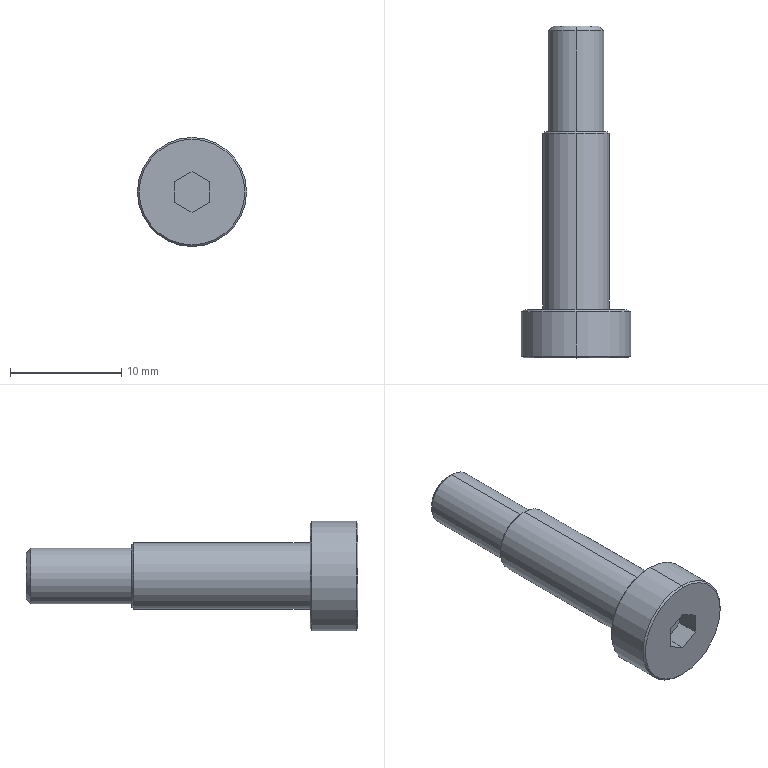Part | SolidWorks | features ICE 2, Chamfer 1, Extrusion 1, StudWizard 1 | 1 solid | 25 faces | box 9.8 x 29.8 x 9.8 mm | volume 943.251 mm3 | plane 11 | cone 8 | cylinder 6 | commonest cylinder face diameters 5 x2 6 x2 9.8 x2
STEP:
#1=CARTESIAN_POINT('',(0.,0.,-4.75));
#2=VERTEX_POINT('',#1);
#3=CARTESIAN_POINT('',(0.,0.,4.75));
#4=VERTEX_POINT('',#3);
#5=CARTESIAN_POINT('',(0.,0.,0.));
#6=DIRECTION('',(0.,-1.,0.));
#7=DIRECTION('',(0.,0.,1.));
#8=AXIS2_PLACEMENT_3D('',#5,#6,#7);
#9=CIRCLE('',#8,4.75);
#10=EDGE_CURVE('',#2,#4,#9,.T.);
#11=ORIENTED_EDGE('',*,*,#10,.F.);
#12=CARTESIAN_POINT('',(0.,0.15,-4.9));
#13=VERTEX_POINT('',#12);
#14=CARTESIAN_POINT('',(0.,0.15,-4.9));
#15=DIRECTION('',(0.,0.7071,-0.7071));
#16=VECTOR('',#15,1000.);
#17=LINE('',#14,#16);
#18=EDGE_CURVE('',#2,#13,#17,.T.);
#19=ORIENTED_EDGE('',*,*,#18,.T.);
#20=CARTESIAN_POINT('',(0.,0.15,4.9));
#21=VERTEX_POINT('',#20);
#22=CARTESIAN_POINT('',(0.,0.15,0.));
#23=DIRECTION('',(0.,1.,0.));
#24=DIRECTION('',(0.,0.,1.));
#25=AXIS2_PLACEMENT_3D('',#22,#23,#24);
#26=CIRCLE('',#25,4.9);
#27=EDGE_CURVE('',#21,#13,#26,.T.);
#28=ORIENTED_EDGE('',*,*,#27,.F.);
#29=CARTESIAN_POINT('',(0.,0.15,4.9));
#30=DIRECTION('',(0.,0.7071,0.7071));
#31=VECTOR('',#30,1000.);
#32=LINE('',#29,#31);
#33=EDGE_CURVE('',#4,#21,#32,.T.);
#34=ORIENTED_EDGE('',*,*,#33,.F.);
#35=EDGE_LOOP('',(#11,#19,#28,#34));
#36=FACE_OUTER_BOUND('',#35,.T.);
#37=CARTESIAN_POINT('',(0.,0.15,0.));
#38=DIRECTION('',(0.,1.,0.));
#39=DIRECTION('',(0.,0.,1.));
#40=AXIS2_PLACEMENT_3D('',#37,#38,#39);
#41=CONICAL_SURFACE('',#40,4.9,0.7854);
#42=ADVANCED_FACE('',(#36),#41,.T.);
#43=CARTESIAN_POINT('',(0.,4.3,4.75));
#44=VERTEX_POINT('',#43);
#45=CARTESIAN_POINT('',(0.,4.3,-4.75));
#46=VERTEX_POINT('',#45);
#47=CARTESIAN_POINT('',(0.,4.3,0.));
#48=DIRECTION('',(0.,1.,0.));
#49=DIRECTION('',(0.,0.,1.));
#50=AXIS2_PLACEMENT_3D('',#47,#48,#49);
#51=CIRCLE('',#50,4.75);
#52=EDGE_CURVE('',#44,#46,#51,.T.);
#53=ORIENTED_EDGE('',*,*,#52,.F.);
#54=CARTESIAN_POINT('',(0.,4.15,4.9));
#55=VERTEX_POINT('',#54);
#56=CARTESIAN_POINT('',(0.,4.3,4.75));
#57=DIRECTION('',(0.,-0.7071,0.7071));
#58=VECTOR('',#57,1000.);
#59=LINE('',#56,#58);
#60=EDGE_CURVE('',#44,#55,#59,.T.);
#61=ORIENTED_EDGE('',*,*,#60,.T.);
#62=CARTESIAN_POINT('',(0.,4.15,-4.9));
#63=VERTEX_POINT('',#62);
#64=CARTESIAN_POINT('',(0.,4.15,0.));
#65=DIRECTION('',(0.,-1.,0.));
#66=DIRECTION('',(0.,0.,1.));
#67=AXIS2_PLACEMENT_3D('',#64,#65,#66);
#68=CIRCLE('',#67,4.9);
#69=EDGE_CURVE('',#63,#55,#68,.T.);
#70=ORIENTED_EDGE('',*,*,#69,.F.);
#71=CARTESIAN_POINT('',(0.,4.3,-4.75));
#72=DIRECTION('',(0.,-0.7071,-0.7071));
#73=VECTOR('',#72,1000.);
#74=LINE('',#71,#73);
#75=EDGE_CURVE('',#46,#63,#74,.T.);
#76=ORIENTED_EDGE('',*,*,#75,.F.);
#77=EDGE_LOOP('',(#53,#61,#70,#76));
#78=FACE_OUTER_BOUND('',#77,.T.);
#79=CARTESIAN_POINT('',(0.,4.3,0.));
#80=DIRECTION('',(0.,-1.,0.));
#81=DIRECTION('',(0.,0.,-1.));
#82=AXIS2_PLACEMENT_3D('',#79,#80,#81);
#83=CONICAL_SURFACE('',#82,4.75,0.7854);
#84=ADVANCED_FACE('',(#78),#83,.T.);
#85=CARTESIAN_POINT('',(0.,20.3,2.85));
#86=VERTEX_POINT('',#85);
#87=CARTESIAN_POINT('',(0.,20.3,-2.85));
#88=VERTEX_POINT('',#87);
#89=CARTESIAN_POINT('',(0.,20.3,0.));
#90=DIRECTION('',(0.,1.,0.));
#91=DIRECTION('',(0.,0.,1.));
#92=AXIS2_PLACEMENT_3D('',#89,#90,#91);
#93=CIRCLE('',#92,2.85);
#94=EDGE_CURVE('',#86,#88,#93,.T.);
#95=ORIENTED_EDGE('',*,*,#94,.F.);
#96=CARTESIAN_POINT('',(0.,20.15,3.));
#97=VERTEX_POINT('',#96);
#98=CARTESIAN_POINT('',(0.,20.3,2.85));
#99=DIRECTION('',(0.,-0.7071,0.7071));
#100=VECTOR('',#99,1000.);
#101=LINE('',#98,#100);
#102=EDGE_CURVE('',#86,#97,#101,.T.);
#103=ORIENTED_EDGE('',*,*,#102,.T.);
#104=CARTESIAN_POINT('',(0.,20.15,-3.));
#105=VERTEX_POINT('',#104);
#106=CARTESIAN_POINT('',(0.,20.15,0.));
#107=DIRECTION('',(0.,-1.,0.));
#108=DIRECTION('',(0.,0.,1.));
#109=AXIS2_PLACEMENT_3D('',#106,#107,#108);
#110=CIRCLE('',#109,3.);
#111=EDGE_CURVE('',#105,#97,#110,.T.);
#112=ORIENTED_EDGE('',*,*,#111,.F.);
#113=CARTESIAN_POINT('',(0.,20.3,-2.85));
#114=DIRECTION('',(0.,-0.7071,-0.7071));
#115=VECTOR('',#114,1000.);
#116=LINE('',#113,#115);
#117=EDGE_CURVE('',#88,#105,#116,.T.);
#118=ORIENTED_EDGE('',*,*,#117,.F.);
#119=EDGE_LOOP('',(#95,#103,#112,#118));
#120=FACE_OUTER_BOUND('',#119,.T.);
#121=CARTESIAN_POINT('',(0.,20.3,0.));
#122=DIRECTION('',(0.,-1.,0.));
#123=DIRECTION('',(0.,0.,-1.));
#124=AXIS2_PLACEMENT_3D('',#121,#122,#123);
#125=CONICAL_SURFACE('',#124,2.85,0.7854);
#126=ADVANCED_FACE('',(#120),#125,.T.);
#127=CARTESIAN_POINT('',(0.,29.367,-2.5));
#128=VERTEX_POINT('',#127);
#129=CARTESIAN_POINT('',(0.,29.367,2.5));
#130=VERTEX_POINT('',#129);
#131=CARTESIAN_POINT('',(0.,29.367,0.));
#132=DIRECTION('',(0.,-1.,0.));
#133=DIRECTION('',(0.,0.,-1.));
#134=AXIS2_PLACEMENT_3D('',#131,#132,#133);
#135=CIRCLE('',#134,2.5);
#136=EDGE_CURVE('',#128,#130,#135,.T.);
#137=ORIENTED_EDGE('',*,*,#136,.T.);
#138=CARTESIAN_POINT('',(0.,20.3,2.5));
#139=VERTEX_POINT('',#138);
#140=CARTESIAN_POINT('',(0.,20.3,2.5));
#141=DIRECTION('',(0.,-1.,0.));
#142=VECTOR('',#141,1000.);
#143=LINE('',#140,#142);
#144=EDGE_CURVE('',#130,#139,#143,.T.);
#145=ORIENTED_EDGE('',*,*,#144,.T.);
#146=CARTESIAN_POINT('',(0.,20.3,-2.5));
#147=VERTEX_POINT('',#146);
#148=CARTESIAN_POINT('',(0.,20.3,0.));
#149=DIRECTION('',(0.,-1.,0.));
#150=DIRECTION('',(0.,0.,-1.));
#151=AXIS2_PLACEMENT_3D('',#148,#149,#150);
#152=CIRCLE('',#151,2.5);
#153=EDGE_CURVE('',#147,#139,#152,.T.);
#154=ORIENTED_EDGE('',*,*,#153,.F.);
#155=CARTESIAN_POINT('',(0.,20.3,-2.5));
#156=DIRECTION('',(0.,-1.,0.));
#157=VECTOR('',#156,1000.);
#158=LINE('',#155,#157);
#159=EDGE_CURVE('',#128,#147,#158,.T.);
#160=ORIENTED_EDGE('',*,*,#159,.F.);
#161=EDGE_LOOP('',(#137,#145,#154,#160));
#162=FACE_OUTER_BOUND('',#161,.T.);
#163=CARTESIAN_POINT('',(0.,20.3,0.));
#164=DIRECTION('',(0.,-1.,0.));
#165=DIRECTION('',(0.,0.,-1.));
#166=AXIS2_PLACEMENT_3D('',#163,#164,#165);
#167=CYLINDRICAL_SURFACE('',#166,2.5);
#168=ADVANCED_FACE('',(#162),#167,.T.);
#169=CARTESIAN_POINT('',(0.,29.8,-2.067));
#170=VERTEX_POINT('',#169);
#171=CARTESIAN_POINT('',(0.,29.8,2.067));
#172=VERTEX_POINT('',#171);
#173=CARTESIAN_POINT('',(0.,29.8,0.));
#174=DIRECTION('',(0.,-1.,0.));
#175=DIRECTION('',(0.,0.,-1.));
#176=AXIS2_PLACEMENT_3D('',#173,#174,#175);
#177=CIRCLE('',#176,2.067);
#178=EDGE_CURVE('',#170,#172,#177,.T.);
#179=ORIENTED_EDGE('',*,*,#178,.T.);
#180=CARTESIAN_POINT('',(0.,29.367,2.5));
#181=DIRECTION('',(0.,-0.7071,0.7071));
#182=VECTOR('',#181,1000.);
#183=LINE('',#180,#182);
#184=EDGE_CURVE('',#172,#130,#183,.T.);
#185=ORIENTED_EDGE('',*,*,#184,.T.);
#186=ORIENTED_EDGE('',*,*,#136,.F.);
#187=CARTESIAN_POINT('',(0.,29.367,-2.5));
#188=DIRECTION('',(0.,-0.7071,-0.7071));
#189=VECTOR('',#188,1000.);
#190=LINE('',#187,#189);
#191=EDGE_CURVE('',#170,#128,#190,.T.);
#192=ORIENTED_EDGE('',*,*,#191,.F.);
#193=EDGE_LOOP('',(#179,#185,#186,#192));
#194=FACE_OUTER_BOUND('',#193,.T.);
#195=CARTESIAN_POINT('',(0.,29.367,0.));
#196=DIRECTION('',(0.,-1.,0.));
#197=DIRECTION('',(0.,0.,-1.));
#198=AXIS2_PLACEMENT_3D('',#195,#196,#197);
#199=CONICAL_SURFACE('',#198,2.5,0.7854);
#200=ADVANCED_FACE('',(#194),#199,.T.);
#201=ORIENTED_EDGE('',*,*,#111,.T.);
#202=CARTESIAN_POINT('',(0.,4.3,3.));
#203=VERTEX_POINT('',#202);
#204=CARTESIAN_POINT('',(0.,20.3,3.));
#205=DIRECTION('',(0.,-1.,0.));
#206=VECTOR('',#205,1000.);
#207=LINE('',#204,#206);
#208=EDGE_CURVE('',#97,#203,#207,.T.);
#209=ORIENTED_EDGE('',*,*,#208,.T.);
#210=CARTESIAN_POINT('',(0.,4.3,-3.));
#211=VERTEX_POINT('',#210);
#212=CARTESIAN_POINT('',(0.,4.3,0.));
#213=DIRECTION('',(0.,1.,0.));
#214=DIRECTION('',(0.,0.,1.));
#215=AXIS2_PLACEMENT_3D('',#212,#213,#214);
#216=CIRCLE('',#215,3.);
#217=EDGE_CURVE('',#203,#211,#216,.T.);
#218=ORIENTED_EDGE('',*,*,#217,.T.);
#219=CARTESIAN_POINT('',(0.,20.3,-3.));
#220=DIRECTION('',(0.,-1.,0.));
#221=VECTOR('',#220,1000.);
#222=LINE('',#219,#221);
#223=EDGE_CURVE('',#105,#211,#222,.T.);
#224=ORIENTED_EDGE('',*,*,#223,.F.);
#225=EDGE_LOOP('',(#201,#209,#218,#224));
#226=FACE_OUTER_BOUND('',#225,.T.);
#227=CARTESIAN_POINT('',(0.,20.3,0.));
#228=DIRECTION('',(0.,-1.,0.));
#229=DIRECTION('',(0.,0.,-1.));
#230=AXIS2_PLACEMENT_3D('',#227,#228,#229);
#231=CYLINDRICAL_SURFACE('',#230,3.);
#232=ADVANCED_FACE('',(#226),#231,.T.);
#233=ORIENTED_EDGE('',*,*,#69,.T.);
#234=CARTESIAN_POINT('',(0.,4.3,4.9));
#235=DIRECTION('',(0.,-1.,0.));
#236=VECTOR('',#235,1000.);
#237=LINE('',#234,#236);
#238=EDGE_CURVE('',#55,#21,#237,.T.);
#239=ORIENTED_EDGE('',*,*,#238,.T.);
#240=ORIENTED_EDGE('',*,*,#27,.T.);
#241=CARTESIAN_POINT('',(0.,4.3,-4.9));
#242=DIRECTION('',(0.,-1.,0.));
#243=VECTOR('',#242,1000.);
#244=LINE('',#241,#243);
#245=EDGE_CURVE('',#63,#13,#244,.T.);
#246=ORIENTED_EDGE('',*,*,#245,.F.);
#247=EDGE_LOOP('',(#233,#239,#240,#246));
#248=FACE_OUTER_BOUND('',#247,.T.);
#249=CARTESIAN_POINT('',(0.,4.3,0.));
#250=DIRECTION('',(0.,-1.,0.));
#251=DIRECTION('',(0.,0.,-1.));
#252=AXIS2_PLACEMENT_3D('',#249,#250,#251);
#253=CYLINDRICAL_SURFACE('',#252,4.9);
#254=ADVANCED_FACE('',(#248),#253,.T.);
#255=ORIENTED_EDGE('',*,*,#238,.F.);
#256=CARTESIAN_POINT('',(0.,4.15,0.));
#257=DIRECTION('',(0.,-1.,0.));
#258=DIRECTION('',(0.,0.,1.));
#259=AXIS2_PLACEMENT_3D('',#256,#257,#258);
#260=CIRCLE('',#259,4.9);
#261=EDGE_CURVE('',#55,#63,#260,.T.);
#262=ORIENTED_EDGE('',*,*,#261,.T.);
#263=ORIENTED_EDGE('',*,*,#245,.T.);
#264=CARTESIAN_POINT('',(0.,0.15,0.));
#265=DIRECTION('',(0.,1.,0.));
#266=DIRECTION('',(0.,0.,1.));
#267=AXIS2_PLACEMENT_3D('',#264,#265,#266);
#268=CIRCLE('',#267,4.9);
#269=EDGE_CURVE('',#13,#21,#268,.T.);
#270=ORIENTED_EDGE('',*,*,#269,.T.);
#271=EDGE_LOOP('',(#255,#262,#263,#270));
#272=FACE_OUTER_BOUND('',#271,.T.);
#273=CARTESIAN_POINT('',(0.,4.3,0.));
#274=DIRECTION('',(0.,-1.,0.));
#275=DIRECTION('',(0.,0.,-1.));
#276=AXIS2_PLACEMENT_3D('',#273,#274,#275);
#277=CYLINDRICAL_SURFACE('',#276,4.9);
#278=ADVANCED_FACE('',(#272),#277,.T.);
#279=CARTESIAN_POINT('',(0.,4.3,0.));
#280=DIRECTION('',(0.,1.,0.));
#281=DIRECTION('',(0.,0.,1.));
#282=AXIS2_PLACEMENT_3D('',#279,#280,#281);
#283=CIRCLE('',#282,4.75);
#284=EDGE_CURVE('',#46,#44,#283,.T.);
#285=ORIENTED_EDGE('',*,*,#284,.T.);
#286=ORIENTED_EDGE('',*,*,#52,.T.);
#287=EDGE_LOOP('',(#285,#286));
#288=FACE_OUTER_BOUND('',#287,.T.);
#289=CARTESIAN_POINT('',(0.,4.3,0.));
#290=DIRECTION('',(0.,1.,0.));
#291=DIRECTION('',(0.,0.,1.));
#292=AXIS2_PLACEMENT_3D('',#289,#290,#291);
#293=CIRCLE('',#292,3.);
#294=EDGE_CURVE('',#211,#203,#293,.T.);
#295=ORIENTED_EDGE('',*,*,#294,.F.);
#296=ORIENTED_EDGE('',*,*,#217,.F.);
#297=EDGE_LOOP('',(#295,#296));
#298=FACE_BOUND('',#297,.T.);
#299=CARTESIAN_POINT('',(0.,4.3,0.));
#300=DIRECTION('',(0.,1.,0.));
#301=DIRECTION('',(0.,0.,1.));
#302=AXIS2_PLACEMENT_3D('',#299,#300,#301);
#303=PLANE('',#302);
#304=ADVANCED_FACE('',(#288,#298),#303,.T.);
#305=CARTESIAN_POINT('',(0.,0.,0.));
#306=DIRECTION('',(0.,-1.,0.));
#307=DIRECTION('',(0.,0.,1.));
#308=AXIS2_PLACEMENT_3D('',#305,#306,#307);
#309=CIRCLE('',#308,4.75);
#310=EDGE_CURVE('',#4,#2,#309,.T.);
#311=ORIENTED_EDGE('',*,*,#310,.T.);
#312=ORIENTED_EDGE('',*,*,#10,.T.);
#313=EDGE_LOOP('',(#311,#312));
#314=FACE_OUTER_BOUND('',#313,.T.);
#315=CARTESIAN_POINT('',(0.,0.,1.848));
#316=VERTEX_POINT('',#315);
#317=CARTESIAN_POINT('',(-1.6,0.,0.9238));
#318=VERTEX_POINT('',#317);
#319=CARTESIAN_POINT('',(0.,0.,1.848));
#320=DIRECTION('',(-0.866,0.,-0.5));
#321=VECTOR('',#320,1000.);
#322=LINE('',#319,#321);
#323=EDGE_CURVE('',#316,#318,#322,.T.);
#324=ORIENTED_EDGE('',*,*,#323,.F.);
#325=CARTESIAN_POINT('',(1.6,0.,0.9238));
#326=VERTEX_POINT('',#325);
#327=CARTESIAN_POINT('',(1.6,0.,0.9238));
#328=DIRECTION('',(-0.866,0.,0.5));
#329=VECTOR('',#328,1000.);
#330=LINE('',#327,#329);
#331=EDGE_CURVE('',#326,#316,#330,.T.);
#332=ORIENTED_EDGE('',*,*,#331,.F.);
#333=CARTESIAN_POINT('',(1.6,0.,-0.9238));
#334=VERTEX_POINT('',#333);
#335=CARTESIAN_POINT('',(1.6,0.,-0.9238));
#336=DIRECTION('',(0.,0.,1.));
#337=VECTOR('',#336,1000.);
#338=LINE('',#335,#337);
#339=EDGE_CURVE('',#334,#326,#338,.T.);
#340=ORIENTED_EDGE('',*,*,#339,.F.);
#341=CARTESIAN_POINT('',(0.,0.,-1.848));
#342=VERTEX_POINT('',#341);
#343=CARTESIAN_POINT('',(0.,0.,-1.848));
#344=DIRECTION('',(0.866,0.,0.5));
#345=VECTOR('',#344,1000.);
#346=LINE('',#343,#345);
#347=EDGE_CURVE('',#342,#334,#346,.T.);
#348=ORIENTED_EDGE('',*,*,#347,.F.);
#349=CARTESIAN_POINT('',(-1.6,0.,-0.9238));
#350=VERTEX_POINT('',#349);
#351=CARTESIAN_POINT('',(-1.6,0.,-0.9238));
#352=DIRECTION('',(0.866,0.,-0.5));
#353=VECTOR('',#352,1000.);
#354=LINE('',#351,#353);
#355=EDGE_CURVE('',#350,#342,#354,.T.);
#356=ORIENTED_EDGE('',*,*,#355,.F.);
#357=CARTESIAN_POINT('',(-1.6,0.,0.9238));
#358=DIRECTION('',(0.,0.,-1.));
#359=VECTOR('',#358,1000.);
#360=LINE('',#357,#359);
#361=EDGE_CURVE('',#318,#350,#360,.T.);
#362=ORIENTED_EDGE('',*,*,#361,.F.);
#363=EDGE_LOOP('',(#324,#332,#340,#348,#356,#362));
#364=FACE_BOUND('',#363,.T.);
#365=CARTESIAN_POINT('',(0.,0.,0.));
#366=DIRECTION('',(0.,1.,0.));
#367=DIRECTION('',(0.,0.,1.));
#368=AXIS2_PLACEMENT_3D('',#365,#366,#367);
#369=PLANE('',#368);
#370=ADVANCED_FACE('',(#314,#364),#369,.F.);
#371=ORIENTED_EDGE('',*,*,#208,.F.);
#372=CARTESIAN_POINT('',(0.,20.15,0.));
#373=DIRECTION('',(0.,-1.,0.));
#374=DIRECTION('',(0.,0.,1.));
#375=AXIS2_PLACEMENT_3D('',#372,#373,#374);
#376=CIRCLE('',#375,3.);
#377=EDGE_CURVE('',#97,#105,#376,.T.);
#378=ORIENTED_EDGE('',*,*,#377,.T.);
#379=ORIENTED_EDGE('',*,*,#223,.T.);
#380=ORIENTED_EDGE('',*,*,#294,.T.);
#381=EDGE_LOOP('',(#371,#378,#379,#380));
#382=FACE_OUTER_BOUND('',#381,.T.);
#383=CARTESIAN_POINT('',(0.,20.3,0.));
#384=DIRECTION('',(0.,-1.,0.));
#385=DIRECTION('',(0.,0.,-1.));
#386=AXIS2_PLACEMENT_3D('',#383,#384,#385);
#387=CYLINDRICAL_SURFACE('',#386,3.);
#388=ADVANCED_FACE('',(#382),#387,.T.);
#389=CARTESIAN_POINT('',(0.,20.3,0.));
#390=DIRECTION('',(0.,1.,0.));
#391=DIRECTION('',(0.,0.,1.));
#392=AXIS2_PLACEMENT_3D('',#389,#390,#391);
#393=CIRCLE('',#392,2.85);
#394=EDGE_CURVE('',#88,#86,#393,.T.);
#395=ORIENTED_EDGE('',*,*,#394,.T.);
#396=ORIENTED_EDGE('',*,*,#94,.T.);
#397=EDGE_LOOP('',(#395,#396));
#398=FACE_OUTER_BOUND('',#397,.T.);
#399=ORIENTED_EDGE('',*,*,#153,.T.);
#400=CARTESIAN_POINT('',(0.,20.3,0.));
#401=DIRECTION('',(0.,-1.,0.));
#402=DIRECTION('',(0.,0.,-1.));
#403=AXIS2_PLACEMENT_3D('',#400,#401,#402);
#404=CIRCLE('',#403,2.5);
#405=EDGE_CURVE('',#139,#147,#404,.T.);
#406=ORIENTED_EDGE('',*,*,#405,.T.);
#407=EDGE_LOOP('',(#399,#406));
#408=FACE_BOUND('',#407,.T.);
#409=CARTESIAN_POINT('',(0.,20.3,0.));
#410=DIRECTION('',(0.,1.,0.));
#411=DIRECTION('',(0.,0.,1.));
#412=AXIS2_PLACEMENT_3D('',#409,#410,#411);
#413=PLANE('',#412);
#414=ADVANCED_FACE('',(#398,#408),#413,.T.);
#415=ORIENTED_EDGE('',*,*,#178,.F.);
#416=CARTESIAN_POINT('',(0.,29.8,0.));
#417=DIRECTION('',(0.,-1.,0.));
#418=DIRECTION('',(0.,0.,-1.));
#419=AXIS2_PLACEMENT_3D('',#416,#417,#418);
#420=CIRCLE('',#419,2.067);
#421=EDGE_CURVE('',#172,#170,#420,.T.);
#422=ORIENTED_EDGE('',*,*,#421,.F.);
#423=EDGE_LOOP('',(#415,#422));
#424=FACE_OUTER_BOUND('',#423,.T.);
#425=CARTESIAN_POINT('',(2.067,29.8,0.));
#426=DIRECTION('',(0.,1.,0.));
#427=DIRECTION('',(0.,0.,1.));
#428=AXIS2_PLACEMENT_3D('',#425,#426,#427);
#429=PLANE('',#428);
#430=ADVANCED_FACE('',(#424),#429,.T.);
#431=ORIENTED_EDGE('',*,*,#184,.F.);
#432=ORIENTED_EDGE('',*,*,#421,.T.);
#433=ORIENTED_EDGE('',*,*,#191,.T.);
#434=CARTESIAN_POINT('',(0.,29.367,0.));
#435=DIRECTION('',(0.,-1.,0.));
#436=DIRECTION('',(0.,0.,-1.));
#437=AXIS2_PLACEMENT_3D('',#434,#435,#436);
#438=CIRCLE('',#437,2.5);
#439=EDGE_CURVE('',#130,#128,#438,.T.);
#440=ORIENTED_EDGE('',*,*,#439,.F.);
#441=EDGE_LOOP('',(#431,#432,#433,#440));
#442=FACE_OUTER_BOUND('',#441,.T.);
#443=CARTESIAN_POINT('',(0.,29.367,0.));
#444=DIRECTION('',(0.,-1.,0.));
#445=DIRECTION('',(0.,0.,-1.));
#446=AXIS2_PLACEMENT_3D('',#443,#444,#445);
#447=CONICAL_SURFACE('',#446,2.5,0.7854);
#448=ADVANCED_FACE('',(#442),#447,.T.);
#449=ORIENTED_EDGE('',*,*,#144,.F.);
#450=ORIENTED_EDGE('',*,*,#439,.T.);
#451=ORIENTED_EDGE('',*,*,#159,.T.);
#452=ORIENTED_EDGE('',*,*,#405,.F.);
#453=EDGE_LOOP('',(#449,#450,#451,#452));
#454=FACE_OUTER_BOUND('',#453,.T.);
#455=CARTESIAN_POINT('',(0.,20.3,0.));
#456=DIRECTION('',(0.,-1.,0.));
#457=DIRECTION('',(0.,0.,-1.));
#458=AXIS2_PLACEMENT_3D('',#455,#456,#457);
#459=CYLINDRICAL_SURFACE('',#458,2.5);
#460=ADVANCED_FACE('',(#454),#459,.T.);
#461=ORIENTED_EDGE('',*,*,#331,.T.);
#462=CARTESIAN_POINT('',(0.,2.,1.848));
#463=VERTEX_POINT('',#462);
#464=CARTESIAN_POINT('',(0.,2.,1.848));
#465=DIRECTION('',(0.,-1.,0.));
#466=VECTOR('',#465,1000.);
#467=LINE('',#464,#466);
#468=EDGE_CURVE('',#463,#316,#467,.T.);
#469=ORIENTED_EDGE('',*,*,#468,.F.);
#470=CARTESIAN_POINT('',(1.6,2.,0.9238));
#471=VERTEX_POINT('',#470);
#472=CARTESIAN_POINT('',(1.6,2.,0.9238));
#473=DIRECTION('',(-0.866,0.,0.5));
#474=VECTOR('',#473,1000.);
#475=LINE('',#472,#474);
#476=EDGE_CURVE('',#471,#463,#475,.T.);
#477=ORIENTED_EDGE('',*,*,#476,.F.);
#478=CARTESIAN_POINT('',(1.6,2.,0.9238));
#479=DIRECTION('',(0.,-1.,0.));
#480=VECTOR('',#479,1000.);
#481=LINE('',#478,#480);
#482=EDGE_CURVE('',#471,#326,#481,.T.);
#483=ORIENTED_EDGE('',*,*,#482,.T.);
#484=EDGE_LOOP('',(#461,#469,#477,#483));
#485=FACE_OUTER_BOUND('',#484,.T.);
#486=CARTESIAN_POINT('',(1.6,2.,0.9238));
#487=DIRECTION('',(0.5,0.,0.866));
#488=DIRECTION('',(0.866,0.,-0.5));
#489=AXIS2_PLACEMENT_3D('',#486,#487,#488);
#490=PLANE('',#489);
#491=ADVANCED_FACE('',(#485),#490,.F.);
#492=ORIENTED_EDGE('',*,*,#339,.T.);
#493=ORIENTED_EDGE('',*,*,#482,.F.);
#494=CARTESIAN_POINT('',(1.6,2.,-0.9238));
#495=VERTEX_POINT('',#494);
#496=CARTESIAN_POINT('',(1.6,2.,-0.9238));
#497=DIRECTION('',(0.,0.,1.));
#498=VECTOR('',#497,1000.);
#499=LINE('',#496,#498);
#500=EDGE_CURVE('',#495,#471,#499,.T.);
#501=ORIENTED_EDGE('',*,*,#500,.F.);
#502=CARTESIAN_POINT('',(1.6,2.,-0.9238));
#503=DIRECTION('',(0.,-1.,0.));
#504=VECTOR('',#503,1000.);
#505=LINE('',#502,#504);
#506=EDGE_CURVE('',#495,#334,#505,.T.);
#507=ORIENTED_EDGE('',*,*,#506,.T.);
#508=EDGE_LOOP('',(#492,#493,#501,#507));
#509=FACE_OUTER_BOUND('',#508,.T.);
#510=CARTESIAN_POINT('',(1.6,2.,-0.9238));
#511=DIRECTION('',(1.,0.,0.));
#512=DIRECTION('',(0.,0.,-1.));
#513=AXIS2_PLACEMENT_3D('',#510,#511,#512);
#514=PLANE('',#513);
#515=ADVANCED_FACE('',(#509),#514,.F.);
#516=ORIENTED_EDGE('',*,*,#347,.T.);
#517=ORIENTED_EDGE('',*,*,#506,.F.);
#518=CARTESIAN_POINT('',(0.,2.,-1.848));
#519=VERTEX_POINT('',#518);
#520=CARTESIAN_POINT('',(0.,2.,-1.848));
#521=DIRECTION('',(0.866,0.,0.5));
#522=VECTOR('',#521,1000.);
#523=LINE('',#520,#522);
#524=EDGE_CURVE('',#519,#495,#523,.T.);
#525=ORIENTED_EDGE('',*,*,#524,.F.);
#526=CARTESIAN_POINT('',(0.,2.,-1.848));
#527=DIRECTION('',(0.,-1.,0.));
#528=VECTOR('',#527,1000.);
#529=LINE('',#526,#528);
#530=EDGE_CURVE('',#519,#342,#529,.T.);
#531=ORIENTED_EDGE('',*,*,#530,.T.);
#532=EDGE_LOOP('',(#516,#517,#525,#531));
#533=FACE_OUTER_BOUND('',#532,.T.);
#534=CARTESIAN_POINT('',(0.,2.,-1.848));
#535=DIRECTION('',(0.5,0.,-0.866));
#536=DIRECTION('',(-0.866,0.,-0.5));
#537=AXIS2_PLACEMENT_3D('',#534,#535,#536);
#538=PLANE('',#537);
#539=ADVANCED_FACE('',(#533),#538,.F.);
#540=ORIENTED_EDGE('',*,*,#355,.T.);
#541=ORIENTED_EDGE('',*,*,#530,.F.);
#542=CARTESIAN_POINT('',(-1.6,2.,-0.9238));
#543=VERTEX_POINT('',#542);
#544=CARTESIAN_POINT('',(-1.6,2.,-0.9238));
#545=DIRECTION('',(0.866,0.,-0.5));
#546=VECTOR('',#545,1000.);
#547=LINE('',#544,#546);
#548=EDGE_CURVE('',#543,#519,#547,.T.);
#549=ORIENTED_EDGE('',*,*,#548,.F.);
#550=CARTESIAN_POINT('',(-1.6,2.,-0.9238));
#551=DIRECTION('',(0.,-1.,0.));
#552=VECTOR('',#551,1000.);
#553=LINE('',#550,#552);
#554=EDGE_CURVE('',#543,#350,#553,.T.);
#555=ORIENTED_EDGE('',*,*,#554,.T.);
#556=EDGE_LOOP('',(#540,#541,#549,#555));
#557=FACE_OUTER_BOUND('',#556,.T.);
#558=CARTESIAN_POINT('',(-1.6,2.,-0.9238));
#559=DIRECTION('',(-0.5,0.,-0.866));
#560=DIRECTION('',(-0.866,0.,0.5));
#561=AXIS2_PLACEMENT_3D('',#558,#559,#560);
#562=PLANE('',#561);
#563=ADVANCED_FACE('',(#557),#562,.F.);
#564=ORIENTED_EDGE('',*,*,#361,.T.);
#565=ORIENTED_EDGE('',*,*,#554,.F.);
#566=CARTESIAN_POINT('',(-1.6,2.,0.9238));
#567=VERTEX_POINT('',#566);
#568=CARTESIAN_POINT('',(-1.6,2.,0.9238));
#569=DIRECTION('',(0.,0.,-1.));
#570=VECTOR('',#569,1000.);
#571=LINE('',#568,#570);
#572=EDGE_CURVE('',#567,#543,#571,.T.);
#573=ORIENTED_EDGE('',*,*,#572,.F.);
#574=CARTESIAN_POINT('',(-1.6,2.,0.9238));
#575=DIRECTION('',(0.,-1.,0.));
#576=VECTOR('',#575,1000.);
#577=LINE('',#574,#576);
#578=EDGE_CURVE('',#567,#318,#577,.T.);
#579=ORIENTED_EDGE('',*,*,#578,.T.);
#580=EDGE_LOOP('',(#564,#565,#573,#579));
#581=FACE_OUTER_BOUND('',#580,.T.);
#582=CARTESIAN_POINT('',(-1.6,2.,0.9238));
#583=DIRECTION('',(-1.,0.,0.));
#584=DIRECTION('',(0.,0.,1.));
#585=AXIS2_PLACEMENT_3D('',#582,#583,#584);
#586=PLANE('',#585);
#587=ADVANCED_FACE('',(#581),#586,.F.);
#588=ORIENTED_EDGE('',*,*,#323,.T.);
#589=ORIENTED_EDGE('',*,*,#578,.F.);
#590=CARTESIAN_POINT('',(0.,2.,1.848));
#591=DIRECTION('',(-0.866,0.,-0.5));
#592=VECTOR('',#591,1000.);
#593=LINE('',#590,#592);
#594=EDGE_CURVE('',#463,#567,#593,.T.);
#595=ORIENTED_EDGE('',*,*,#594,.F.);
#596=ORIENTED_EDGE('',*,*,#468,.T.);
#597=EDGE_LOOP('',(#588,#589,#595,#596));
#598=FACE_OUTER_BOUND('',#597,.T.);
#599=CARTESIAN_POINT('',(0.,2.,1.848));
#600=DIRECTION('',(-0.5,0.,0.866));
#601=DIRECTION('',(0.866,0.,0.5));
#602=AXIS2_PLACEMENT_3D('',#599,#600,#601);
#603=PLANE('',#602);
#604=ADVANCED_FACE('',(#598),#603,.F.);
#605=ORIENTED_EDGE('',*,*,#476,.T.);
#606=ORIENTED_EDGE('',*,*,#594,.T.);
#607=ORIENTED_EDGE('',*,*,#572,.T.);
#608=ORIENTED_EDGE('',*,*,#548,.T.);
#609=ORIENTED_EDGE('',*,*,#524,.T.);
#610=ORIENTED_EDGE('',*,*,#500,.T.);
#611=EDGE_LOOP('',(#605,#606,#607,#608,#609,#610));
#612=FACE_OUTER_BOUND('',#611,.T.);
#613=CARTESIAN_POINT('',(0.,2.,0.));
#614=DIRECTION('',(0.,-1.,0.));
#615=DIRECTION('',(0.,0.,-1.));
#616=AXIS2_PLACEMENT_3D('',#613,#614,#615);
#617=PLANE('',#616);
#618=ADVANCED_FACE('',(#612),#617,.T.);
#619=ORIENTED_EDGE('',*,*,#102,.F.);
#620=ORIENTED_EDGE('',*,*,#394,.F.);
#621=ORIENTED_EDGE('',*,*,#117,.T.);
#622=ORIENTED_EDGE('',*,*,#377,.F.);
#623=EDGE_LOOP('',(#619,#620,#621,#622));
#624=FACE_OUTER_BOUND('',#623,.T.);
#625=CARTESIAN_POINT('',(0.,20.3,0.));
#626=DIRECTION('',(0.,-1.,0.));
#627=DIRECTION('',(0.,0.,-1.));
#628=AXIS2_PLACEMENT_3D('',#625,#626,#627);
#629=CONICAL_SURFACE('',#628,2.85,0.7854);
#630=ADVANCED_FACE('',(#624),#629,.T.);
#631=ORIENTED_EDGE('',*,*,#60,.F.);
#632=ORIENTED_EDGE('',*,*,#284,.F.);
#633=ORIENTED_EDGE('',*,*,#75,.T.);
#634=ORIENTED_EDGE('',*,*,#261,.F.);
#635=EDGE_LOOP('',(#631,#632,#633,#634));
#636=FACE_OUTER_BOUND('',#635,.T.);
#637=CARTESIAN_POINT('',(0.,4.3,0.));
#638=DIRECTION('',(0.,-1.,0.));
#639=DIRECTION('',(0.,0.,-1.));
#640=AXIS2_PLACEMENT_3D('',#637,#638,#639);
#641=CONICAL_SURFACE('',#640,4.75,0.7854);
#642=ADVANCED_FACE('',(#636),#641,.T.);
#643=ORIENTED_EDGE('',*,*,#18,.F.);
#644=ORIENTED_EDGE('',*,*,#310,.F.);
#645=ORIENTED_EDGE('',*,*,#33,.T.);
#646=ORIENTED_EDGE('',*,*,#269,.F.);
#647=EDGE_LOOP('',(#643,#644,#645,#646));
#648=FACE_OUTER_BOUND('',#647,.T.);
#649=CARTESIAN_POINT('',(0.,0.15,0.));
#650=DIRECTION('',(0.,1.,0.));
#651=DIRECTION('',(0.,0.,1.));
#652=AXIS2_PLACEMENT_3D('',#649,#650,#651);
#653=CONICAL_SURFACE('',#652,4.9,0.7854);
#654=ADVANCED_FACE('',(#648),#653,.T.);
#655=CLOSED_SHELL('',(#42,#84,#126,#168,#200,#232,#254,#278,#304,#370,#388,#414,#430,#448,#460,#491,#515,#539,#563,#587,#604,#618,#630,#642,#654));
#656=MANIFOLD_SOLID_BREP('',#655);
#657=CARTESIAN_POINT('',(0.,0.,0.));
#658=DIRECTION('',(0.,0.,1.));
#659=DIRECTION('',(1.,0.,0.));
#660=AXIS2_PLACEMENT_3D('',#657,#658,#659);
#661=(LENGTH_UNIT()NAMED_UNIT(*)SI_UNIT(.MILLI.,.METRE.));
#662=UNCERTAINTY_MEASURE_WITH_UNIT(LENGTH_MEASURE(0.00001),#661,'','');
#663=(NAMED_UNIT(*)PLANE_ANGLE_UNIT()SI_UNIT($,.RADIAN.));
#664=(NAMED_UNIT(*)SI_UNIT($,.STERADIAN.)SOLID_ANGLE_UNIT());
#665=(GEOMETRIC_REPRESENTATION_CONTEXT(3)GLOBAL_UNCERTAINTY_ASSIGNED_CONTEXT((#662))GLOBAL_UNIT_ASSIGNED_CONTEXT((#661,#663,#664))REPRESENTATION_CONTEXT('',''));
#666=ADVANCED_BREP_SHAPE_REPRESENTATION('',(#656,#660),#665);